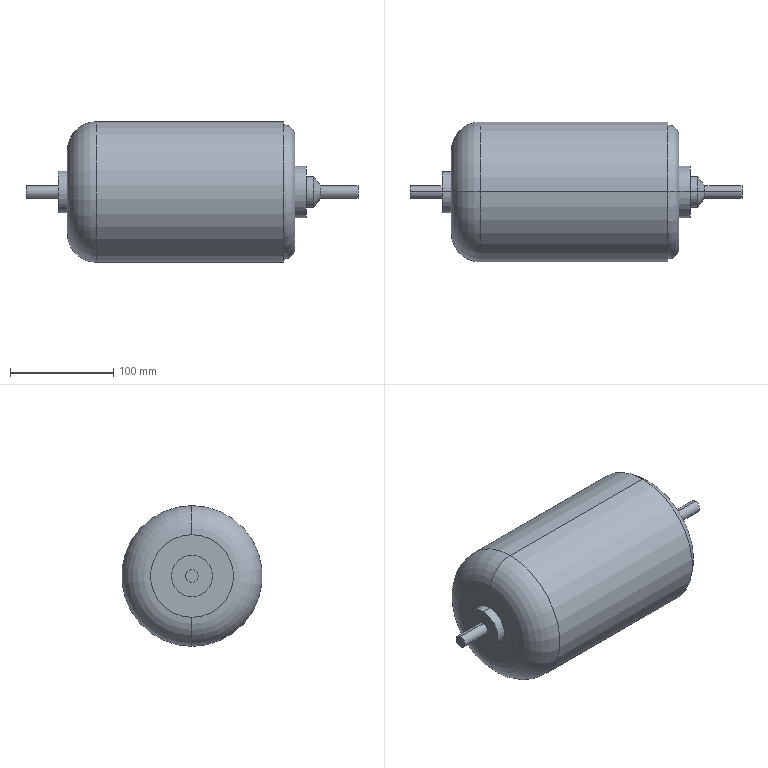Part | NX | features BREP 1 | 1 solid | 35 faces | box 321 x 136 x 136 mm | volume 3154531 mm3 | cylinder 16 | plane 13 | torus 4 | cone 2 | commonest cylinder face diameters 3 x4 12 x4 30 x2 40 x2 50 x2 136 x2
STEP:
#1=CARTESIAN_POINT('',(184.,0.,20.));
#2=VERTEX_POINT('',#1);
#3=CARTESIAN_POINT('',(184.,0.,-20.));
#4=VERTEX_POINT('',#3);
#5=CARTESIAN_POINT('',(184.,0.,0.));
#6=DIRECTION('',(-1.,0.,0.));
#7=DIRECTION('',(0.,0.,1.));
#8=AXIS2_PLACEMENT_3D('',#5,#6,#7);
#9=CIRCLE('',#8,20.);
#10=EDGE_CURVE('',#2,#4,#9,.T.);
#11=ORIENTED_EDGE('',*,*,#10,.T.);
#12=CARTESIAN_POINT('',(175.,0.,-20.));
#13=VERTEX_POINT('',#12);
#14=CARTESIAN_POINT('',(144.,0.,-20.));
#15=DIRECTION('',(-1.,0.,0.));
#16=VECTOR('',#15,1000.);
#17=LINE('',#14,#16);
#18=EDGE_CURVE('',#4,#13,#17,.T.);
#19=ORIENTED_EDGE('',*,*,#18,.T.);
#20=CARTESIAN_POINT('',(175.,0.,20.));
#21=VERTEX_POINT('',#20);
#22=CARTESIAN_POINT('',(175.,0.,0.));
#23=DIRECTION('',(-1.,0.,0.));
#24=DIRECTION('',(0.,0.,1.));
#25=AXIS2_PLACEMENT_3D('',#22,#23,#24);
#26=CIRCLE('',#25,20.);
#27=EDGE_CURVE('',#21,#13,#26,.T.);
#28=ORIENTED_EDGE('',*,*,#27,.F.);
#29=CARTESIAN_POINT('',(144.,0.,20.));
#30=DIRECTION('',(-1.,0.,0.));
#31=VECTOR('',#30,1000.);
#32=LINE('',#29,#31);
#33=EDGE_CURVE('',#2,#21,#32,.T.);
#34=ORIENTED_EDGE('',*,*,#33,.F.);
#35=EDGE_LOOP('',(#11,#19,#28,#34));
#36=FACE_BOUND('',#35,.T.);
#37=CARTESIAN_POINT('',(144.,0.,0.));
#38=DIRECTION('',(-1.,0.,0.));
#39=DIRECTION('',(0.,0.,-1.));
#40=AXIS2_PLACEMENT_3D('',#37,#38,#39);
#41=CYLINDRICAL_SURFACE('',#40,20.);
#42=ADVANCED_FACE('',(#36),#41,.T.);
#43=CARTESIAN_POINT('',(175.,0.,6.));
#44=VERTEX_POINT('',#43);
#45=CARTESIAN_POINT('',(175.,0.,-6.));
#46=VERTEX_POINT('',#45);
#47=CARTESIAN_POINT('',(175.,0.,0.));
#48=DIRECTION('',(-1.,0.,0.));
#49=DIRECTION('',(0.,0.,1.));
#50=AXIS2_PLACEMENT_3D('',#47,#48,#49);
#51=CIRCLE('',#50,6.);
#52=EDGE_CURVE('',#44,#46,#51,.T.);
#53=ORIENTED_EDGE('',*,*,#52,.T.);
#54=CARTESIAN_POINT('',(144.,0.,-6.));
#55=VERTEX_POINT('',#54);
#56=CARTESIAN_POINT('',(144.,0.,-6.));
#57=DIRECTION('',(-1.,0.,0.));
#58=VECTOR('',#57,1000.);
#59=LINE('',#56,#58);
#60=EDGE_CURVE('',#46,#55,#59,.T.);
#61=ORIENTED_EDGE('',*,*,#60,.T.);
#62=CARTESIAN_POINT('',(144.,0.,6.));
#63=VERTEX_POINT('',#62);
#64=CARTESIAN_POINT('',(144.,0.,0.));
#65=DIRECTION('',(-1.,0.,0.));
#66=DIRECTION('',(0.,0.,1.));
#67=AXIS2_PLACEMENT_3D('',#64,#65,#66);
#68=CIRCLE('',#67,6.);
#69=EDGE_CURVE('',#63,#55,#68,.T.);
#70=ORIENTED_EDGE('',*,*,#69,.F.);
#71=CARTESIAN_POINT('',(144.,0.,6.));
#72=DIRECTION('',(-1.,0.,0.));
#73=VECTOR('',#72,1000.);
#74=LINE('',#71,#73);
#75=EDGE_CURVE('',#44,#63,#74,.T.);
#76=ORIENTED_EDGE('',*,*,#75,.F.);
#77=EDGE_LOOP('',(#53,#61,#70,#76));
#78=FACE_BOUND('',#77,.T.);
#79=CARTESIAN_POINT('',(156.,5.809,-1.5));
#80=VERTEX_POINT('',#79);
#81=CARTESIAN_POINT('',(164.,5.809,-1.5));
#82=VERTEX_POINT('',#81);
#83=CARTESIAN_POINT('',(144.,5.809,-1.5));
#84=DIRECTION('',(1.,0.,0.));
#85=VECTOR('',#84,1000.);
#86=LINE('',#83,#85);
#87=EDGE_CURVE('',#80,#82,#86,.T.);
#88=ORIENTED_EDGE('',*,*,#87,.T.);
#89=CARTESIAN_POINT('',(164.,5.809,1.5));
#90=VERTEX_POINT('',#89);
#91=CARTESIAN_POINT('',(164.,5.809,-1.5));
#92=CARTESIAN_POINT('',(164.398,5.809,-1.5));
#93=CARTESIAN_POINT('',(165.172,5.906,-1.175));
#94=CARTESIAN_POINT('',(165.664,6.047,-0.002103));
#95=CARTESIAN_POINT('',(165.173,5.906,1.175));
#96=CARTESIAN_POINT('',(164.398,5.809,1.5));
#97=CARTESIAN_POINT('',(164.,5.809,1.5));
#98=B_SPLINE_CURVE_WITH_KNOTS('',3,(#91,#92,#93,#94,#95,#96,#97),.UNSPECIFIED.,.F.,.F.,(4,1,1,1,4),(0.,0.001177,0.002353,0.00353,0.004707),.UNSPECIFIED.);
#99=EDGE_CURVE('',#82,#90,#98,.T.);
#100=ORIENTED_EDGE('',*,*,#99,.T.);
#101=CARTESIAN_POINT('',(156.,5.809,1.5));
#102=VERTEX_POINT('',#101);
#103=CARTESIAN_POINT('',(144.,5.809,1.5));
#104=DIRECTION('',(-1.,0.,0.));
#105=VECTOR('',#104,1000.);
#106=LINE('',#103,#105);
#107=EDGE_CURVE('',#90,#102,#106,.T.);
#108=ORIENTED_EDGE('',*,*,#107,.T.);
#109=CARTESIAN_POINT('',(156.,5.809,1.5));
#110=CARTESIAN_POINT('',(155.602,5.809,1.5));
#111=CARTESIAN_POINT('',(154.828,5.906,1.175));
#112=CARTESIAN_POINT('',(154.336,6.047,0.002103));
#113=CARTESIAN_POINT('',(154.827,5.906,-1.175));
#114=CARTESIAN_POINT('',(155.602,5.809,-1.5));
#115=CARTESIAN_POINT('',(156.,5.809,-1.5));
#116=B_SPLINE_CURVE_WITH_KNOTS('',3,(#109,#110,#111,#112,#113,#114,#115),.UNSPECIFIED.,.F.,.F.,(4,1,1,1,4),(0.,0.001177,0.002353,0.00353,0.004707),.UNSPECIFIED.);
#117=EDGE_CURVE('',#102,#80,#116,.T.);
#118=ORIENTED_EDGE('',*,*,#117,.T.);
#119=EDGE_LOOP('',(#88,#100,#108,#118));
#120=FACE_BOUND('',#119,.T.);
#121=CARTESIAN_POINT('',(144.,0.,0.));
#122=DIRECTION('',(-1.,0.,0.));
#123=DIRECTION('',(0.,0.,-1.));
#124=AXIS2_PLACEMENT_3D('',#121,#122,#123);
#125=CYLINDRICAL_SURFACE('',#124,6.);
#126=ADVANCED_FACE('',(#78,#120),#125,.T.);
#127=CARTESIAN_POINT('',(465.,0.,6.));
#128=VERTEX_POINT('',#127);
#129=CARTESIAN_POINT('',(465.,0.,-6.));
#130=VERTEX_POINT('',#129);
#131=CARTESIAN_POINT('',(465.,0.,0.));
#132=DIRECTION('',(-1.,0.,0.));
#133=DIRECTION('',(0.,0.,1.));
#134=AXIS2_PLACEMENT_3D('',#131,#132,#133);
#135=CIRCLE('',#134,6.);
#136=EDGE_CURVE('',#128,#130,#135,.T.);
#137=ORIENTED_EDGE('',*,*,#136,.T.);
#138=CARTESIAN_POINT('',(429.,0.,-6.));
#139=VERTEX_POINT('',#138);
#140=CARTESIAN_POINT('',(144.,0.,-6.));
#141=DIRECTION('',(-1.,0.,0.));
#142=VECTOR('',#141,1000.);
#143=LINE('',#140,#142);
#144=EDGE_CURVE('',#130,#139,#143,.T.);
#145=ORIENTED_EDGE('',*,*,#144,.T.);
#146=CARTESIAN_POINT('',(429.,0.,6.));
#147=VERTEX_POINT('',#146);
#148=CARTESIAN_POINT('',(429.,0.,0.));
#149=DIRECTION('',(-1.,0.,0.));
#150=DIRECTION('',(0.,0.,1.));
#151=AXIS2_PLACEMENT_3D('',#148,#149,#150);
#152=CIRCLE('',#151,6.);
#153=EDGE_CURVE('',#147,#139,#152,.T.);
#154=ORIENTED_EDGE('',*,*,#153,.F.);
#155=CARTESIAN_POINT('',(144.,0.,6.));
#156=DIRECTION('',(-1.,0.,0.));
#157=VECTOR('',#156,1000.);
#158=LINE('',#155,#157);
#159=EDGE_CURVE('',#128,#147,#158,.T.);
#160=ORIENTED_EDGE('',*,*,#159,.F.);
#161=EDGE_LOOP('',(#137,#145,#154,#160));
#162=FACE_BOUND('',#161,.T.);
#163=CARTESIAN_POINT('',(444.,5.809,-1.5));
#164=VERTEX_POINT('',#163);
#165=CARTESIAN_POINT('',(452.,5.809,-1.5));
#166=VERTEX_POINT('',#165);
#167=CARTESIAN_POINT('',(144.,5.809,-1.5));
#168=DIRECTION('',(1.,0.,0.));
#169=VECTOR('',#168,1000.);
#170=LINE('',#167,#169);
#171=EDGE_CURVE('',#164,#166,#170,.T.);
#172=ORIENTED_EDGE('',*,*,#171,.T.);
#173=CARTESIAN_POINT('',(452.,5.809,1.5));
#174=VERTEX_POINT('',#173);
#175=CARTESIAN_POINT('',(452.,5.809,-1.5));
#176=CARTESIAN_POINT('',(452.398,5.809,-1.5));
#177=CARTESIAN_POINT('',(453.172,5.906,-1.175));
#178=CARTESIAN_POINT('',(453.664,6.047,-0.002103));
#179=CARTESIAN_POINT('',(453.173,5.906,1.175));
#180=CARTESIAN_POINT('',(452.398,5.809,1.5));
#181=CARTESIAN_POINT('',(452.,5.809,1.5));
#182=B_SPLINE_CURVE_WITH_KNOTS('',3,(#175,#176,#177,#178,#179,#180,#181),.UNSPECIFIED.,.F.,.F.,(4,1,1,1,4),(0.,0.001177,0.002353,0.00353,0.004707),.UNSPECIFIED.);
#183=EDGE_CURVE('',#166,#174,#182,.T.);
#184=ORIENTED_EDGE('',*,*,#183,.T.);
#185=CARTESIAN_POINT('',(444.,5.809,1.5));
#186=VERTEX_POINT('',#185);
#187=CARTESIAN_POINT('',(144.,5.809,1.5));
#188=DIRECTION('',(-1.,0.,0.));
#189=VECTOR('',#188,1000.);
#190=LINE('',#187,#189);
#191=EDGE_CURVE('',#174,#186,#190,.T.);
#192=ORIENTED_EDGE('',*,*,#191,.T.);
#193=CARTESIAN_POINT('',(444.,5.809,1.5));
#194=CARTESIAN_POINT('',(443.602,5.809,1.5));
#195=CARTESIAN_POINT('',(442.828,5.906,1.175));
#196=CARTESIAN_POINT('',(442.336,6.047,0.002103));
#197=CARTESIAN_POINT('',(442.827,5.906,-1.175));
#198=CARTESIAN_POINT('',(443.602,5.809,-1.5));
#199=CARTESIAN_POINT('',(444.,5.809,-1.5));
#200=B_SPLINE_CURVE_WITH_KNOTS('',3,(#193,#194,#195,#196,#197,#198,#199),.UNSPECIFIED.,.F.,.F.,(4,1,1,1,4),(0.,0.001177,0.002353,0.00353,0.004707),.UNSPECIFIED.);
#201=EDGE_CURVE('',#186,#164,#200,.T.);
#202=ORIENTED_EDGE('',*,*,#201,.T.);
#203=EDGE_LOOP('',(#172,#184,#192,#202));
#204=FACE_BOUND('',#203,.T.);
#205=CARTESIAN_POINT('',(144.,0.,0.));
#206=DIRECTION('',(-1.,0.,0.));
#207=DIRECTION('',(0.,0.,-1.));
#208=AXIS2_PLACEMENT_3D('',#205,#206,#207);
#209=CYLINDRICAL_SURFACE('',#208,6.);
#210=ADVANCED_FACE('',(#162,#204),#209,.T.);
#211=ORIENTED_EDGE('',*,*,#153,.T.);
#212=CARTESIAN_POINT('',(422.,0.,-15.));
#213=VERTEX_POINT('',#212);
#214=CARTESIAN_POINT('',(429.,0.,-6.));
#215=DIRECTION('',(-0.6139,0.,-0.7894));
#216=VECTOR('',#215,1000.);
#217=LINE('',#214,#216);
#218=EDGE_CURVE('',#139,#213,#217,.T.);
#219=ORIENTED_EDGE('',*,*,#218,.T.);
#220=CARTESIAN_POINT('',(422.,0.,15.));
#221=VERTEX_POINT('',#220);
#222=CARTESIAN_POINT('',(422.,0.,0.));
#223=DIRECTION('',(-1.,0.,0.));
#224=DIRECTION('',(0.,0.,1.));
#225=AXIS2_PLACEMENT_3D('',#222,#223,#224);
#226=CIRCLE('',#225,15.);
#227=EDGE_CURVE('',#221,#213,#226,.T.);
#228=ORIENTED_EDGE('',*,*,#227,.F.);
#229=CARTESIAN_POINT('',(429.,0.,6.));
#230=DIRECTION('',(-0.6139,0.,0.7894));
#231=VECTOR('',#230,1000.);
#232=LINE('',#229,#231);
#233=EDGE_CURVE('',#147,#221,#232,.T.);
#234=ORIENTED_EDGE('',*,*,#233,.F.);
#235=EDGE_LOOP('',(#211,#219,#228,#234));
#236=FACE_BOUND('',#235,.T.);
#237=CARTESIAN_POINT('',(429.,0.,0.));
#238=DIRECTION('',(-1.,0.,0.));
#239=DIRECTION('',(0.,0.,-1.));
#240=AXIS2_PLACEMENT_3D('',#237,#238,#239);
#241=CONICAL_SURFACE('',#240,6.,0.9098);
#242=ADVANCED_FACE('',(#236),#241,.T.);
#243=ORIENTED_EDGE('',*,*,#227,.T.);
#244=CARTESIAN_POINT('',(415.,0.,-15.));
#245=VERTEX_POINT('',#244);
#246=CARTESIAN_POINT('',(144.,0.,-15.));
#247=DIRECTION('',(-1.,0.,0.));
#248=VECTOR('',#247,1000.);
#249=LINE('',#246,#248);
#250=EDGE_CURVE('',#213,#245,#249,.T.);
#251=ORIENTED_EDGE('',*,*,#250,.T.);
#252=CARTESIAN_POINT('',(415.,0.,15.));
#253=VERTEX_POINT('',#252);
#254=CARTESIAN_POINT('',(415.,0.,0.));
#255=DIRECTION('',(-1.,0.,0.));
#256=DIRECTION('',(0.,0.,1.));
#257=AXIS2_PLACEMENT_3D('',#254,#255,#256);
#258=CIRCLE('',#257,15.);
#259=EDGE_CURVE('',#253,#245,#258,.T.);
#260=ORIENTED_EDGE('',*,*,#259,.F.);
#261=CARTESIAN_POINT('',(144.,0.,15.));
#262=DIRECTION('',(-1.,0.,0.));
#263=VECTOR('',#262,1000.);
#264=LINE('',#261,#263);
#265=EDGE_CURVE('',#221,#253,#264,.T.);
#266=ORIENTED_EDGE('',*,*,#265,.F.);
#267=EDGE_LOOP('',(#243,#251,#260,#266));
#268=FACE_BOUND('',#267,.T.);
#269=CARTESIAN_POINT('',(144.,0.,0.));
#270=DIRECTION('',(-1.,0.,0.));
#271=DIRECTION('',(0.,0.,-1.));
#272=AXIS2_PLACEMENT_3D('',#269,#270,#271);
#273=CYLINDRICAL_SURFACE('',#272,15.);
#274=ADVANCED_FACE('',(#268),#273,.T.);
#275=CARTESIAN_POINT('',(415.,0.,25.));
#276=VERTEX_POINT('',#275);
#277=CARTESIAN_POINT('',(415.,0.,-25.));
#278=VERTEX_POINT('',#277);
#279=CARTESIAN_POINT('',(415.,0.,0.));
#280=DIRECTION('',(-1.,0.,0.));
#281=DIRECTION('',(0.,0.,1.));
#282=AXIS2_PLACEMENT_3D('',#279,#280,#281);
#283=CIRCLE('',#282,25.);
#284=EDGE_CURVE('',#276,#278,#283,.T.);
#285=ORIENTED_EDGE('',*,*,#284,.T.);
#286=CARTESIAN_POINT('',(404.,0.,-25.));
#287=VERTEX_POINT('',#286);
#288=CARTESIAN_POINT('',(144.,0.,-25.));
#289=DIRECTION('',(-1.,0.,0.));
#290=VECTOR('',#289,1000.);
#291=LINE('',#288,#290);
#292=EDGE_CURVE('',#278,#287,#291,.T.);
#293=ORIENTED_EDGE('',*,*,#292,.T.);
#294=CARTESIAN_POINT('',(404.,0.,25.));
#295=VERTEX_POINT('',#294);
#296=CARTESIAN_POINT('',(404.,0.,0.));
#297=DIRECTION('',(-1.,0.,0.));
#298=DIRECTION('',(0.,0.,1.));
#299=AXIS2_PLACEMENT_3D('',#296,#297,#298);
#300=CIRCLE('',#299,25.);
#301=EDGE_CURVE('',#295,#287,#300,.T.);
#302=ORIENTED_EDGE('',*,*,#301,.F.);
#303=CARTESIAN_POINT('',(144.,0.,25.));
#304=DIRECTION('',(-1.,0.,0.));
#305=VECTOR('',#304,1000.);
#306=LINE('',#303,#305);
#307=EDGE_CURVE('',#276,#295,#306,.T.);
#308=ORIENTED_EDGE('',*,*,#307,.F.);
#309=EDGE_LOOP('',(#285,#293,#302,#308));
#310=FACE_BOUND('',#309,.T.);
#311=CARTESIAN_POINT('',(144.,0.,0.));
#312=DIRECTION('',(-1.,0.,0.));
#313=DIRECTION('',(0.,0.,-1.));
#314=AXIS2_PLACEMENT_3D('',#311,#312,#313);
#315=CYLINDRICAL_SURFACE('',#314,25.);
#316=ADVANCED_FACE('',(#310),#315,.T.);
#317=CARTESIAN_POINT('',(404.,0.,54.));
#318=VERTEX_POINT('',#317);
#319=CARTESIAN_POINT('',(404.,0.,-54.));
#320=VERTEX_POINT('',#319);
#321=CARTESIAN_POINT('',(404.,0.,0.));
#322=DIRECTION('',(-1.,0.,0.));
#323=DIRECTION('',(0.,0.,1.));
#324=AXIS2_PLACEMENT_3D('',#321,#322,#323);
#325=CIRCLE('',#324,54.);
#326=EDGE_CURVE('',#318,#320,#325,.T.);
#327=ORIENTED_EDGE('',*,*,#326,.T.);
#328=CARTESIAN_POINT('',(393.,0.,-65.));
#329=VERTEX_POINT('',#328);
#330=CARTESIAN_POINT('',(393.,0.,-54.));
#331=DIRECTION('',(0.,1.,0.));
#332=DIRECTION('',(0.,0.,1.));
#333=AXIS2_PLACEMENT_3D('',#330,#331,#332);
#334=CIRCLE('',#333,11.);
#335=EDGE_CURVE('',#320,#329,#334,.T.);
#336=ORIENTED_EDGE('',*,*,#335,.T.);
#337=CARTESIAN_POINT('',(393.,0.,65.));
#338=VERTEX_POINT('',#337);
#339=CARTESIAN_POINT('',(393.,0.,0.));
#340=DIRECTION('',(-1.,0.,0.));
#341=DIRECTION('',(0.,0.,1.));
#342=AXIS2_PLACEMENT_3D('',#339,#340,#341);
#343=CIRCLE('',#342,65.);
#344=EDGE_CURVE('',#338,#329,#343,.T.);
#345=ORIENTED_EDGE('',*,*,#344,.F.);
#346=CARTESIAN_POINT('',(393.,0.,54.));
#347=DIRECTION('',(0.,-1.,0.));
#348=DIRECTION('',(0.,0.,-1.));
#349=AXIS2_PLACEMENT_3D('',#346,#347,#348);
#350=CIRCLE('',#349,11.);
#351=EDGE_CURVE('',#318,#338,#350,.T.);
#352=ORIENTED_EDGE('',*,*,#351,.F.);
#353=EDGE_LOOP('',(#327,#336,#345,#352));
#354=FACE_BOUND('',#353,.T.);
#355=CARTESIAN_POINT('',(393.,0.,0.));
#356=DIRECTION('',(-1.,0.,0.));
#357=DIRECTION('',(0.,0.,-1.));
#358=AXIS2_PLACEMENT_3D('',#355,#356,#357);
#359=TOROIDAL_SURFACE('',#358,54.,11.);
#360=ADVANCED_FACE('',(#354),#359,.T.);
#361=CARTESIAN_POINT('',(393.,0.,68.));
#362=VERTEX_POINT('',#361);
#363=CARTESIAN_POINT('',(393.,0.,-68.));
#364=VERTEX_POINT('',#363);
#365=CARTESIAN_POINT('',(393.,0.,0.));
#366=DIRECTION('',(-1.,0.,0.));
#367=DIRECTION('',(0.,0.,1.));
#368=AXIS2_PLACEMENT_3D('',#365,#366,#367);
#369=CIRCLE('',#368,68.);
#370=EDGE_CURVE('',#362,#364,#369,.T.);
#371=ORIENTED_EDGE('',*,*,#370,.T.);
#372=CARTESIAN_POINT('',(212.,0.,-68.));
#373=VERTEX_POINT('',#372);
#374=CARTESIAN_POINT('',(144.,0.,-68.));
#375=DIRECTION('',(-1.,0.,0.));
#376=VECTOR('',#375,1000.);
#377=LINE('',#374,#376);
#378=EDGE_CURVE('',#364,#373,#377,.T.);
#379=ORIENTED_EDGE('',*,*,#378,.T.);
#380=CARTESIAN_POINT('',(212.,0.,68.));
#381=VERTEX_POINT('',#380);
#382=CARTESIAN_POINT('',(212.,0.,0.));
#383=DIRECTION('',(-1.,0.,0.));
#384=DIRECTION('',(0.,0.,1.));
#385=AXIS2_PLACEMENT_3D('',#382,#383,#384);
#386=CIRCLE('',#385,68.);
#387=EDGE_CURVE('',#381,#373,#386,.T.);
#388=ORIENTED_EDGE('',*,*,#387,.F.);
#389=CARTESIAN_POINT('',(144.,0.,68.));
#390=DIRECTION('',(-1.,0.,0.));
#391=VECTOR('',#390,1000.);
#392=LINE('',#389,#391);
#393=EDGE_CURVE('',#362,#381,#392,.T.);
#394=ORIENTED_EDGE('',*,*,#393,.F.);
#395=EDGE_LOOP('',(#371,#379,#388,#394));
#396=FACE_BOUND('',#395,.T.);
#397=CARTESIAN_POINT('',(144.,0.,0.));
#398=DIRECTION('',(-1.,0.,0.));
#399=DIRECTION('',(0.,0.,-1.));
#400=AXIS2_PLACEMENT_3D('',#397,#398,#399);
#401=CYLINDRICAL_SURFACE('',#400,68.);
#402=ADVANCED_FACE('',(#396),#401,.T.);
#403=ORIENTED_EDGE('',*,*,#387,.T.);
#404=CARTESIAN_POINT('',(184.,0.,-40.));
#405=VERTEX_POINT('',#404);
#406=CARTESIAN_POINT('',(212.,0.,-40.));
#407=DIRECTION('',(0.,1.,0.));
#408=DIRECTION('',(0.,0.,1.));
#409=AXIS2_PLACEMENT_3D('',#406,#407,#408);
#410=CIRCLE('',#409,28.);
#411=EDGE_CURVE('',#373,#405,#410,.T.);
#412=ORIENTED_EDGE('',*,*,#411,.T.);
#413=CARTESIAN_POINT('',(184.,0.,40.));
#414=VERTEX_POINT('',#413);
#415=CARTESIAN_POINT('',(184.,0.,0.));
#416=DIRECTION('',(-1.,0.,0.));
#417=DIRECTION('',(0.,0.,1.));
#418=AXIS2_PLACEMENT_3D('',#415,#416,#417);
#419=CIRCLE('',#418,40.);
#420=EDGE_CURVE('',#414,#405,#419,.T.);
#421=ORIENTED_EDGE('',*,*,#420,.F.);
#422=CARTESIAN_POINT('',(212.,0.,40.));
#423=DIRECTION('',(0.,-1.,0.));
#424=DIRECTION('',(0.,0.,-1.));
#425=AXIS2_PLACEMENT_3D('',#422,#423,#424);
#426=CIRCLE('',#425,28.);
#427=EDGE_CURVE('',#381,#414,#426,.T.);
#428=ORIENTED_EDGE('',*,*,#427,.F.);
#429=EDGE_LOOP('',(#403,#412,#421,#428));
#430=FACE_BOUND('',#429,.T.);
#431=CARTESIAN_POINT('',(212.,0.,0.));
#432=DIRECTION('',(-1.,0.,0.));
#433=DIRECTION('',(0.,0.,-1.));
#434=AXIS2_PLACEMENT_3D('',#431,#432,#433);
#435=TOROIDAL_SURFACE('',#434,40.,28.);
#436=ADVANCED_FACE('',(#430),#435,.T.);
#437=ORIENTED_EDGE('',*,*,#411,.F.);
#438=CARTESIAN_POINT('',(212.,0.,0.));
#439=DIRECTION('',(-1.,0.,0.));
#440=DIRECTION('',(0.,0.,1.));
#441=AXIS2_PLACEMENT_3D('',#438,#439,#440);
#442=CIRCLE('',#441,68.);
#443=EDGE_CURVE('',#373,#381,#442,.T.);
#444=ORIENTED_EDGE('',*,*,#443,.T.);
#445=ORIENTED_EDGE('',*,*,#427,.T.);
#446=CARTESIAN_POINT('',(184.,0.,0.));
#447=DIRECTION('',(-1.,0.,0.));
#448=DIRECTION('',(0.,0.,1.));
#449=AXIS2_PLACEMENT_3D('',#446,#447,#448);
#450=CIRCLE('',#449,40.);
#451=EDGE_CURVE('',#405,#414,#450,.T.);
#452=ORIENTED_EDGE('',*,*,#451,.F.);
#453=EDGE_LOOP('',(#437,#444,#445,#452));
#454=FACE_BOUND('',#453,.T.);
#455=CARTESIAN_POINT('',(212.,0.,0.));
#456=DIRECTION('',(-1.,0.,0.));
#457=DIRECTION('',(0.,0.,-1.));
#458=AXIS2_PLACEMENT_3D('',#455,#456,#457);
#459=TOROIDAL_SURFACE('',#458,40.,28.);
#460=ADVANCED_FACE('',(#454),#459,.T.);
#461=ORIENTED_EDGE('',*,*,#378,.F.);
#462=CARTESIAN_POINT('',(393.,0.,0.));
#463=DIRECTION('',(-1.,0.,0.));
#464=DIRECTION('',(0.,0.,1.));
#465=AXIS2_PLACEMENT_3D('',#462,#463,#464);
#466=CIRCLE('',#465,68.);
#467=EDGE_CURVE('',#364,#362,#466,.T.);
#468=ORIENTED_EDGE('',*,*,#467,.T.);
#469=ORIENTED_EDGE('',*,*,#393,.T.);
#470=ORIENTED_EDGE('',*,*,#443,.F.);
#471=EDGE_LOOP('',(#461,#468,#469,#470));
#472=FACE_BOUND('',#471,.T.);
#473=CARTESIAN_POINT('',(144.,0.,0.));
#474=DIRECTION('',(-1.,0.,0.));
#475=DIRECTION('',(0.,0.,-1.));
#476=AXIS2_PLACEMENT_3D('',#473,#474,#475);
#477=CYLINDRICAL_SURFACE('',#476,68.);
#478=ADVANCED_FACE('',(#472),#477,.T.);
#479=ORIENTED_EDGE('',*,*,#370,.F.);
#480=ORIENTED_EDGE('',*,*,#467,.F.);
#481=EDGE_LOOP('',(#479,#480));
#482=FACE_BOUND('',#481,.T.);
#483=ORIENTED_EDGE('',*,*,#344,.T.);
#484=CARTESIAN_POINT('',(393.,0.,0.));
#485=DIRECTION('',(-1.,0.,0.));
#486=DIRECTION('',(0.,0.,1.));
#487=AXIS2_PLACEMENT_3D('',#484,#485,#486);
#488=CIRCLE('',#487,65.);
#489=EDGE_CURVE('',#329,#338,#488,.T.);
#490=ORIENTED_EDGE('',*,*,#489,.T.);
#491=EDGE_LOOP('',(#483,#490));
#492=FACE_BOUND('',#491,.T.);
#493=CARTESIAN_POINT('',(393.,68.,0.));
#494=DIRECTION('',(-1.,0.,0.));
#495=DIRECTION('',(0.,0.,-1.));
#496=AXIS2_PLACEMENT_3D('',#493,#494,#495);
#497=PLANE('',#496);
#498=ADVANCED_FACE('',(#482,#492),#497,.F.);
#499=ORIENTED_EDGE('',*,*,#335,.F.);
#500=CARTESIAN_POINT('',(404.,0.,0.));
#501=DIRECTION('',(-1.,0.,0.));
#502=DIRECTION('',(0.,0.,1.));
#503=AXIS2_PLACEMENT_3D('',#500,#501,#502);
#504=CIRCLE('',#503,54.);
#505=EDGE_CURVE('',#320,#318,#504,.T.);
#506=ORIENTED_EDGE('',*,*,#505,.T.);
#507=ORIENTED_EDGE('',*,*,#351,.T.);
#508=ORIENTED_EDGE('',*,*,#489,.F.);
#509=EDGE_LOOP('',(#499,#506,#507,#508));
#510=FACE_BOUND('',#509,.T.);
#511=CARTESIAN_POINT('',(393.,0.,0.));
#512=DIRECTION('',(-1.,0.,0.));
#513=DIRECTION('',(0.,0.,-1.));
#514=AXIS2_PLACEMENT_3D('',#511,#512,#513);
#515=TOROIDAL_SURFACE('',#514,54.,11.);
#516=ADVANCED_FACE('',(#510),#515,.T.);
#517=ORIENTED_EDGE('',*,*,#326,.F.);
#518=ORIENTED_EDGE('',*,*,#505,.F.);
#519=EDGE_LOOP('',(#517,#518));
#520=FACE_BOUND('',#519,.T.);
#521=ORIENTED_EDGE('',*,*,#301,.T.);
#522=CARTESIAN_POINT('',(404.,0.,0.));
#523=DIRECTION('',(-1.,0.,0.));
#524=DIRECTION('',(0.,0.,1.));
#525=AXIS2_PLACEMENT_3D('',#522,#523,#524);
#526=CIRCLE('',#525,25.);
#527=EDGE_CURVE('',#287,#295,#526,.T.);
#528=ORIENTED_EDGE('',*,*,#527,.T.);
#529=EDGE_LOOP('',(#521,#528));
#530=FACE_BOUND('',#529,.T.);
#531=CARTESIAN_POINT('',(404.,54.,0.));
#532=DIRECTION('',(-1.,0.,0.));
#533=DIRECTION('',(0.,0.,-1.));
#534=AXIS2_PLACEMENT_3D('',#531,#532,#533);
#535=PLANE('',#534);
#536=ADVANCED_FACE('',(#520,#530),#535,.F.);
#537=ORIENTED_EDGE('',*,*,#292,.F.);
#538=CARTESIAN_POINT('',(415.,0.,0.));
#539=DIRECTION('',(-1.,0.,0.));
#540=DIRECTION('',(0.,0.,1.));
#541=AXIS2_PLACEMENT_3D('',#538,#539,#540);
#542=CIRCLE('',#541,25.);
#543=EDGE_CURVE('',#278,#276,#542,.T.);
#544=ORIENTED_EDGE('',*,*,#543,.T.);
#545=ORIENTED_EDGE('',*,*,#307,.T.);
#546=ORIENTED_EDGE('',*,*,#527,.F.);
#547=EDGE_LOOP('',(#537,#544,#545,#546));
#548=FACE_BOUND('',#547,.T.);
#549=CARTESIAN_POINT('',(144.,0.,0.));
#550=DIRECTION('',(-1.,0.,0.));
#551=DIRECTION('',(0.,0.,-1.));
#552=AXIS2_PLACEMENT_3D('',#549,#550,#551);
#553=CYLINDRICAL_SURFACE('',#552,25.);
#554=ADVANCED_FACE('',(#548),#553,.T.);
#555=ORIENTED_EDGE('',*,*,#284,.F.);
#556=ORIENTED_EDGE('',*,*,#543,.F.);
#557=EDGE_LOOP('',(#555,#556));
#558=FACE_BOUND('',#557,.T.);
#559=ORIENTED_EDGE('',*,*,#259,.T.);
#560=CARTESIAN_POINT('',(415.,0.,0.));
#561=DIRECTION('',(-1.,0.,0.));
#562=DIRECTION('',(0.,0.,1.));
#563=AXIS2_PLACEMENT_3D('',#560,#561,#562);
#564=CIRCLE('',#563,15.);
#565=EDGE_CURVE('',#245,#253,#564,.T.);
#566=ORIENTED_EDGE('',*,*,#565,.T.);
#567=EDGE_LOOP('',(#559,#566));
#568=FACE_BOUND('',#567,.T.);
#569=CARTESIAN_POINT('',(415.,25.,0.));
#570=DIRECTION('',(-1.,0.,0.));
#571=DIRECTION('',(0.,0.,-1.));
#572=AXIS2_PLACEMENT_3D('',#569,#570,#571);
#573=PLANE('',#572);
#574=ADVANCED_FACE('',(#558,#568),#573,.F.);
#575=ORIENTED_EDGE('',*,*,#250,.F.);
#576=CARTESIAN_POINT('',(422.,0.,0.));
#577=DIRECTION('',(-1.,0.,0.));
#578=DIRECTION('',(0.,0.,1.));
#579=AXIS2_PLACEMENT_3D('',#576,#577,#578);
#580=CIRCLE('',#579,15.);
#581=EDGE_CURVE('',#213,#221,#580,.T.);
#582=ORIENTED_EDGE('',*,*,#581,.T.);
#583=ORIENTED_EDGE('',*,*,#265,.T.);
#584=ORIENTED_EDGE('',*,*,#565,.F.);
#585=EDGE_LOOP('',(#575,#582,#583,#584));
#586=FACE_BOUND('',#585,.T.);
#587=CARTESIAN_POINT('',(144.,0.,0.));
#588=DIRECTION('',(-1.,0.,0.));
#589=DIRECTION('',(0.,0.,-1.));
#590=AXIS2_PLACEMENT_3D('',#587,#588,#589);
#591=CYLINDRICAL_SURFACE('',#590,15.);
#592=ADVANCED_FACE('',(#586),#591,.T.);
#593=ORIENTED_EDGE('',*,*,#218,.F.);
#594=CARTESIAN_POINT('',(429.,0.,0.));
#595=DIRECTION('',(-1.,0.,0.));
#596=DIRECTION('',(0.,0.,1.));
#597=AXIS2_PLACEMENT_3D('',#594,#595,#596);
#598=CIRCLE('',#597,6.);
#599=EDGE_CURVE('',#139,#147,#598,.T.);
#600=ORIENTED_EDGE('',*,*,#599,.T.);
#601=ORIENTED_EDGE('',*,*,#233,.T.);
#602=ORIENTED_EDGE('',*,*,#581,.F.);
#603=EDGE_LOOP('',(#593,#600,#601,#602));
#604=FACE_BOUND('',#603,.T.);
#605=CARTESIAN_POINT('',(429.,0.,0.));
#606=DIRECTION('',(-1.,0.,0.));
#607=DIRECTION('',(0.,0.,-1.));
#608=AXIS2_PLACEMENT_3D('',#605,#606,#607);
#609=CONICAL_SURFACE('',#608,6.,0.9098);
#610=ADVANCED_FACE('',(#604),#609,.T.);
#611=ORIENTED_EDGE('',*,*,#144,.F.);
#612=CARTESIAN_POINT('',(465.,0.,0.));
#613=DIRECTION('',(-1.,0.,0.));
#614=DIRECTION('',(0.,0.,1.));
#615=AXIS2_PLACEMENT_3D('',#612,#613,#614);
#616=CIRCLE('',#615,6.);
#617=EDGE_CURVE('',#130,#128,#616,.T.);
#618=ORIENTED_EDGE('',*,*,#617,.T.);
#619=ORIENTED_EDGE('',*,*,#159,.T.);
#620=ORIENTED_EDGE('',*,*,#599,.F.);
#621=EDGE_LOOP('',(#611,#618,#619,#620));
#622=FACE_BOUND('',#621,.T.);
#623=CARTESIAN_POINT('',(144.,0.,0.));
#624=DIRECTION('',(-1.,0.,0.));
#625=DIRECTION('',(0.,0.,-1.));
#626=AXIS2_PLACEMENT_3D('',#623,#624,#625);
#627=CYLINDRICAL_SURFACE('',#626,6.);
#628=ADVANCED_FACE('',(#622),#627,.T.);
#629=ORIENTED_EDGE('',*,*,#136,.F.);
#630=ORIENTED_EDGE('',*,*,#617,.F.);
#631=EDGE_LOOP('',(#629,#630));
#632=FACE_BOUND('',#631,.T.);
#633=CARTESIAN_POINT('',(465.,6.,0.));
#634=DIRECTION('',(-1.,0.,0.));
#635=DIRECTION('',(0.,0.,-1.));
#636=AXIS2_PLACEMENT_3D('',#633,#634,#635);
#637=PLANE('',#636);
#638=ADVANCED_FACE('',(#632),#637,.F.);
#639=ORIENTED_EDGE('',*,*,#69,.T.);
#640=CARTESIAN_POINT('',(144.,0.,0.));
#641=DIRECTION('',(-1.,0.,0.));
#642=DIRECTION('',(0.,0.,1.));
#643=AXIS2_PLACEMENT_3D('',#640,#641,#642);
#644=CIRCLE('',#643,6.);
#645=EDGE_CURVE('',#55,#63,#644,.T.);
#646=ORIENTED_EDGE('',*,*,#645,.T.);
#647=EDGE_LOOP('',(#639,#646));
#648=FACE_BOUND('',#647,.T.);
#649=CARTESIAN_POINT('',(144.,6.,0.));
#650=DIRECTION('',(1.,0.,0.));
#651=DIRECTION('',(0.,0.,-1.));
#652=AXIS2_PLACEMENT_3D('',#649,#650,#651);
#653=PLANE('',#652);
#654=ADVANCED_FACE('',(#648),#653,.F.);
#655=ORIENTED_EDGE('',*,*,#60,.F.);
#656=CARTESIAN_POINT('',(175.,0.,0.));
#657=DIRECTION('',(-1.,0.,0.));
#658=DIRECTION('',(0.,0.,1.));
#659=AXIS2_PLACEMENT_3D('',#656,#657,#658);
#660=CIRCLE('',#659,6.);
#661=EDGE_CURVE('',#46,#44,#660,.T.);
#662=ORIENTED_EDGE('',*,*,#661,.T.);
#663=ORIENTED_EDGE('',*,*,#75,.T.);
#664=ORIENTED_EDGE('',*,*,#645,.F.);
#665=EDGE_LOOP('',(#655,#662,#663,#664));
#666=FACE_BOUND('',#665,.T.);
#667=CARTESIAN_POINT('',(144.,0.,0.));
#668=DIRECTION('',(-1.,0.,0.));
#669=DIRECTION('',(0.,0.,-1.));
#670=AXIS2_PLACEMENT_3D('',#667,#668,#669);
#671=CYLINDRICAL_SURFACE('',#670,6.);
#672=ADVANCED_FACE('',(#666),#671,.T.);
#673=ORIENTED_EDGE('',*,*,#27,.T.);
#674=CARTESIAN_POINT('',(175.,0.,0.));
#675=DIRECTION('',(-1.,0.,0.));
#676=DIRECTION('',(0.,0.,1.));
#677=AXIS2_PLACEMENT_3D('',#674,#675,#676);
#678=CIRCLE('',#677,20.);
#679=EDGE_CURVE('',#13,#21,#678,.T.);
#680=ORIENTED_EDGE('',*,*,#679,.T.);
#681=EDGE_LOOP('',(#673,#680));
#682=FACE_BOUND('',#681,.T.);
#683=ORIENTED_EDGE('',*,*,#52,.F.);
#684=ORIENTED_EDGE('',*,*,#661,.F.);
#685=EDGE_LOOP('',(#683,#684));
#686=FACE_BOUND('',#685,.T.);
#687=CARTESIAN_POINT('',(175.,6.,0.));
#688=DIRECTION('',(1.,0.,0.));
#689=DIRECTION('',(0.,0.,-1.));
#690=AXIS2_PLACEMENT_3D('',#687,#688,#689);
#691=PLANE('',#690);
#692=ADVANCED_FACE('',(#682,#686),#691,.F.);
#693=ORIENTED_EDGE('',*,*,#18,.F.);
#694=CARTESIAN_POINT('',(184.,0.,0.));
#695=DIRECTION('',(-1.,0.,0.));
#696=DIRECTION('',(0.,0.,1.));
#697=AXIS2_PLACEMENT_3D('',#694,#695,#696);
#698=CIRCLE('',#697,20.);
#699=EDGE_CURVE('',#4,#2,#698,.T.);
#700=ORIENTED_EDGE('',*,*,#699,.T.);
#701=ORIENTED_EDGE('',*,*,#33,.T.);
#702=ORIENTED_EDGE('',*,*,#679,.F.);
#703=EDGE_LOOP('',(#693,#700,#701,#702));
#704=FACE_BOUND('',#703,.T.);
#705=CARTESIAN_POINT('',(144.,0.,0.));
#706=DIRECTION('',(-1.,0.,0.));
#707=DIRECTION('',(0.,0.,-1.));
#708=AXIS2_PLACEMENT_3D('',#705,#706,#707);
#709=CYLINDRICAL_SURFACE('',#708,20.);
#710=ADVANCED_FACE('',(#704),#709,.T.);
#711=ORIENTED_EDGE('',*,*,#420,.T.);
#712=ORIENTED_EDGE('',*,*,#451,.T.);
#713=EDGE_LOOP('',(#711,#712));
#714=FACE_BOUND('',#713,.T.);
#715=ORIENTED_EDGE('',*,*,#10,.F.);
#716=ORIENTED_EDGE('',*,*,#699,.F.);
#717=EDGE_LOOP('',(#715,#716));
#718=FACE_BOUND('',#717,.T.);
#719=CARTESIAN_POINT('',(184.,40.,0.));
#720=DIRECTION('',(1.,0.,0.));
#721=DIRECTION('',(0.,0.,-1.));
#722=AXIS2_PLACEMENT_3D('',#719,#720,#721);
#723=PLANE('',#722);
#724=ADVANCED_FACE('',(#714,#718),#723,.F.);
#725=CARTESIAN_POINT('',(444.,4.5,1.5));
#726=VERTEX_POINT('',#725);
#727=CARTESIAN_POINT('',(444.,4.5,1.5));
#728=DIRECTION('',(0.,1.,0.));
#729=VECTOR('',#728,1000.);
#730=LINE('',#727,#729);
#731=EDGE_CURVE('',#726,#186,#730,.T.);
#732=ORIENTED_EDGE('',*,*,#731,.F.);
#733=CARTESIAN_POINT('',(444.,4.5,-1.5));
#734=VERTEX_POINT('',#733);
#735=CARTESIAN_POINT('',(444.,4.5,0.));
#736=DIRECTION('',(0.,1.,0.));
#737=DIRECTION('',(0.,0.,1.));
#738=AXIS2_PLACEMENT_3D('',#735,#736,#737);
#739=CIRCLE('',#738,1.5);
#740=EDGE_CURVE('',#734,#726,#739,.T.);
#741=ORIENTED_EDGE('',*,*,#740,.F.);
#742=CARTESIAN_POINT('',(444.,4.5,-1.5));
#743=DIRECTION('',(0.,1.,0.));
#744=VECTOR('',#743,1000.);
#745=LINE('',#742,#744);
#746=EDGE_CURVE('',#734,#164,#745,.T.);
#747=ORIENTED_EDGE('',*,*,#746,.T.);
#748=ORIENTED_EDGE('',*,*,#201,.F.);
#749=EDGE_LOOP('',(#732,#741,#747,#748));
#750=FACE_BOUND('',#749,.T.);
#751=CARTESIAN_POINT('',(444.,4.5,0.));
#752=DIRECTION('',(0.,1.,0.));
#753=DIRECTION('',(0.,0.,-1.));
#754=AXIS2_PLACEMENT_3D('',#751,#752,#753);
#755=CYLINDRICAL_SURFACE('',#754,1.5);
#756=ADVANCED_FACE('',(#750),#755,.F.);
#757=ORIENTED_EDGE('',*,*,#746,.F.);
#758=CARTESIAN_POINT('',(452.,4.5,-1.5));
#759=VERTEX_POINT('',#758);
#760=CARTESIAN_POINT('',(444.,4.5,-1.5));
#761=DIRECTION('',(-1.,0.,0.));
#762=VECTOR('',#761,1000.);
#763=LINE('',#760,#762);
#764=EDGE_CURVE('',#759,#734,#763,.T.);
#765=ORIENTED_EDGE('',*,*,#764,.F.);
#766=CARTESIAN_POINT('',(452.,4.5,-1.5));
#767=DIRECTION('',(0.,1.,0.));
#768=VECTOR('',#767,1000.);
#769=LINE('',#766,#768);
#770=EDGE_CURVE('',#759,#166,#769,.T.);
#771=ORIENTED_EDGE('',*,*,#770,.T.);
#772=ORIENTED_EDGE('',*,*,#171,.F.);
#773=EDGE_LOOP('',(#757,#765,#771,#772));
#774=FACE_BOUND('',#773,.T.);
#775=CARTESIAN_POINT('',(444.,4.5,-1.5));
#776=DIRECTION('',(0.,0.,-1.));
#777=DIRECTION('',(0.,1.,0.));
#778=AXIS2_PLACEMENT_3D('',#775,#776,#777);
#779=PLANE('',#778);
#780=ADVANCED_FACE('',(#774),#779,.F.);
#781=ORIENTED_EDGE('',*,*,#770,.F.);
#782=CARTESIAN_POINT('',(452.,4.5,1.5));
#783=VERTEX_POINT('',#782);
#784=CARTESIAN_POINT('',(452.,4.5,0.));
#785=DIRECTION('',(0.,1.,0.));
#786=DIRECTION('',(0.,0.,1.));
#787=AXIS2_PLACEMENT_3D('',#784,#785,#786);
#788=CIRCLE('',#787,1.5);
#789=EDGE_CURVE('',#783,#759,#788,.T.);
#790=ORIENTED_EDGE('',*,*,#789,.F.);
#791=CARTESIAN_POINT('',(452.,4.5,1.5));
#792=DIRECTION('',(0.,1.,0.));
#793=VECTOR('',#792,1000.);
#794=LINE('',#791,#793);
#795=EDGE_CURVE('',#783,#174,#794,.T.);
#796=ORIENTED_EDGE('',*,*,#795,.T.);
#797=ORIENTED_EDGE('',*,*,#183,.F.);
#798=EDGE_LOOP('',(#781,#790,#796,#797));
#799=FACE_BOUND('',#798,.T.);
#800=CARTESIAN_POINT('',(452.,4.5,0.));
#801=DIRECTION('',(0.,1.,0.));
#802=DIRECTION('',(0.,0.,-1.));
#803=AXIS2_PLACEMENT_3D('',#800,#801,#802);
#804=CYLINDRICAL_SURFACE('',#803,1.5);
#805=ADVANCED_FACE('',(#799),#804,.F.);
#806=ORIENTED_EDGE('',*,*,#795,.F.);
#807=CARTESIAN_POINT('',(444.,4.5,1.5));
#808=DIRECTION('',(1.,0.,0.));
#809=VECTOR('',#808,1000.);
#810=LINE('',#807,#809);
#811=EDGE_CURVE('',#726,#783,#810,.T.);
#812=ORIENTED_EDGE('',*,*,#811,.F.);
#813=ORIENTED_EDGE('',*,*,#731,.T.);
#814=ORIENTED_EDGE('',*,*,#191,.F.);
#815=EDGE_LOOP('',(#806,#812,#813,#814));
#816=FACE_BOUND('',#815,.T.);
#817=CARTESIAN_POINT('',(444.,4.5,1.5));
#818=DIRECTION('',(0.,0.,1.));
#819=DIRECTION('',(0.,1.,0.));
#820=AXIS2_PLACEMENT_3D('',#817,#818,#819);
#821=PLANE('',#820);
#822=ADVANCED_FACE('',(#816),#821,.F.);
#823=ORIENTED_EDGE('',*,*,#740,.T.);
#824=ORIENTED_EDGE('',*,*,#811,.T.);
#825=ORIENTED_EDGE('',*,*,#789,.T.);
#826=ORIENTED_EDGE('',*,*,#764,.T.);
#827=EDGE_LOOP('',(#823,#824,#825,#826));
#828=FACE_BOUND('',#827,.T.);
#829=CARTESIAN_POINT('',(444.,4.5,0.));
#830=DIRECTION('',(0.,1.,0.));
#831=DIRECTION('',(0.,0.,1.));
#832=AXIS2_PLACEMENT_3D('',#829,#830,#831);
#833=PLANE('',#832);
#834=ADVANCED_FACE('',(#828),#833,.T.);
#835=CARTESIAN_POINT('',(156.,4.5,1.5));
#836=VERTEX_POINT('',#835);
#837=CARTESIAN_POINT('',(156.,4.5,1.5));
#838=DIRECTION('',(0.,1.,0.));
#839=VECTOR('',#838,1000.);
#840=LINE('',#837,#839);
#841=EDGE_CURVE('',#836,#102,#840,.T.);
#842=ORIENTED_EDGE('',*,*,#841,.F.);
#843=CARTESIAN_POINT('',(156.,4.5,-1.5));
#844=VERTEX_POINT('',#843);
#845=CARTESIAN_POINT('',(156.,4.5,0.));
#846=DIRECTION('',(0.,1.,0.));
#847=DIRECTION('',(0.,0.,1.));
#848=AXIS2_PLACEMENT_3D('',#845,#846,#847);
#849=CIRCLE('',#848,1.5);
#850=EDGE_CURVE('',#844,#836,#849,.T.);
#851=ORIENTED_EDGE('',*,*,#850,.F.);
#852=CARTESIAN_POINT('',(156.,4.5,-1.5));
#853=DIRECTION('',(0.,1.,0.));
#854=VECTOR('',#853,1000.);
#855=LINE('',#852,#854);
#856=EDGE_CURVE('',#844,#80,#855,.T.);
#857=ORIENTED_EDGE('',*,*,#856,.T.);
#858=ORIENTED_EDGE('',*,*,#117,.F.);
#859=EDGE_LOOP('',(#842,#851,#857,#858));
#860=FACE_BOUND('',#859,.T.);
#861=CARTESIAN_POINT('',(156.,4.5,0.));
#862=DIRECTION('',(0.,1.,0.));
#863=DIRECTION('',(0.,0.,-1.));
#864=AXIS2_PLACEMENT_3D('',#861,#862,#863);
#865=CYLINDRICAL_SURFACE('',#864,1.5);
#866=ADVANCED_FACE('',(#860),#865,.F.);
#867=ORIENTED_EDGE('',*,*,#856,.F.);
#868=CARTESIAN_POINT('',(164.,4.5,-1.5));
#869=VERTEX_POINT('',#868);
#870=CARTESIAN_POINT('',(156.,4.5,-1.5));
#871=DIRECTION('',(-1.,0.,0.));
#872=VECTOR('',#871,1000.);
#873=LINE('',#870,#872);
#874=EDGE_CURVE('',#869,#844,#873,.T.);
#875=ORIENTED_EDGE('',*,*,#874,.F.);
#876=CARTESIAN_POINT('',(164.,4.5,-1.5));
#877=DIRECTION('',(0.,1.,0.));
#878=VECTOR('',#877,1000.);
#879=LINE('',#876,#878);
#880=EDGE_CURVE('',#869,#82,#879,.T.);
#881=ORIENTED_EDGE('',*,*,#880,.T.);
#882=ORIENTED_EDGE('',*,*,#87,.F.);
#883=EDGE_LOOP('',(#867,#875,#881,#882));
#884=FACE_BOUND('',#883,.T.);
#885=CARTESIAN_POINT('',(156.,4.5,-1.5));
#886=DIRECTION('',(0.,0.,-1.));
#887=DIRECTION('',(0.,1.,0.));
#888=AXIS2_PLACEMENT_3D('',#885,#886,#887);
#889=PLANE('',#888);
#890=ADVANCED_FACE('',(#884),#889,.F.);
#891=ORIENTED_EDGE('',*,*,#880,.F.);
#892=CARTESIAN_POINT('',(164.,4.5,1.5));
#893=VERTEX_POINT('',#892);
#894=CARTESIAN_POINT('',(164.,4.5,0.));
#895=DIRECTION('',(0.,1.,0.));
#896=DIRECTION('',(0.,0.,1.));
#897=AXIS2_PLACEMENT_3D('',#894,#895,#896);
#898=CIRCLE('',#897,1.5);
#899=EDGE_CURVE('',#893,#869,#898,.T.);
#900=ORIENTED_EDGE('',*,*,#899,.F.);
#901=CARTESIAN_POINT('',(164.,4.5,1.5));
#902=DIRECTION('',(0.,1.,0.));
#903=VECTOR('',#902,1000.);
#904=LINE('',#901,#903);
#905=EDGE_CURVE('',#893,#90,#904,.T.);
#906=ORIENTED_EDGE('',*,*,#905,.T.);
#907=ORIENTED_EDGE('',*,*,#99,.F.);
#908=EDGE_LOOP('',(#891,#900,#906,#907));
#909=FACE_BOUND('',#908,.T.);
#910=CARTESIAN_POINT('',(164.,4.5,0.));
#911=DIRECTION('',(0.,1.,0.));
#912=DIRECTION('',(0.,0.,-1.));
#913=AXIS2_PLACEMENT_3D('',#910,#911,#912);
#914=CYLINDRICAL_SURFACE('',#913,1.5);
#915=ADVANCED_FACE('',(#909),#914,.F.);
#916=ORIENTED_EDGE('',*,*,#905,.F.);
#917=CARTESIAN_POINT('',(156.,4.5,1.5));
#918=DIRECTION('',(1.,0.,0.));
#919=VECTOR('',#918,1000.);
#920=LINE('',#917,#919);
#921=EDGE_CURVE('',#836,#893,#920,.T.);
#922=ORIENTED_EDGE('',*,*,#921,.F.);
#923=ORIENTED_EDGE('',*,*,#841,.T.);
#924=ORIENTED_EDGE('',*,*,#107,.F.);
#925=EDGE_LOOP('',(#916,#922,#923,#924));
#926=FACE_BOUND('',#925,.T.);
#927=CARTESIAN_POINT('',(156.,4.5,1.5));
#928=DIRECTION('',(0.,0.,1.));
#929=DIRECTION('',(0.,1.,0.));
#930=AXIS2_PLACEMENT_3D('',#927,#928,#929);
#931=PLANE('',#930);
#932=ADVANCED_FACE('',(#926),#931,.F.);
#933=ORIENTED_EDGE('',*,*,#850,.T.);
#934=ORIENTED_EDGE('',*,*,#921,.T.);
#935=ORIENTED_EDGE('',*,*,#899,.T.);
#936=ORIENTED_EDGE('',*,*,#874,.T.);
#937=EDGE_LOOP('',(#933,#934,#935,#936));
#938=FACE_BOUND('',#937,.T.);
#939=CARTESIAN_POINT('',(156.,4.5,0.));
#940=DIRECTION('',(0.,1.,0.));
#941=DIRECTION('',(0.,0.,1.));
#942=AXIS2_PLACEMENT_3D('',#939,#940,#941);
#943=PLANE('',#942);
#944=ADVANCED_FACE('',(#938),#943,.T.);
#945=CLOSED_SHELL('',(#42,#126,#210,#242,#274,#316,#360,#402,#436,#460,#478,#498,#516,#536,#554,#574,#592,#610,#628,#638,#654,#672,#692,#710,#724,#756,#780,#805,#822,#834,#866,#890,#915,#932,#944));
#946=MANIFOLD_SOLID_BREP('',#945);
#947=(LENGTH_UNIT()NAMED_UNIT(*)SI_UNIT(.MILLI.,.METRE.));
#948=UNCERTAINTY_MEASURE_WITH_UNIT(LENGTH_MEASURE(0.0508),#947,'','');
#949=(NAMED_UNIT(*)PLANE_ANGLE_UNIT()SI_UNIT($,.RADIAN.));
#950=(NAMED_UNIT(*)SI_UNIT($,.STERADIAN.)SOLID_ANGLE_UNIT());
#951=(GEOMETRIC_REPRESENTATION_CONTEXT(3)GLOBAL_UNCERTAINTY_ASSIGNED_CONTEXT((#948))GLOBAL_UNIT_ASSIGNED_CONTEXT((#947,#949,#950))REPRESENTATION_CONTEXT('',''));
#952=ADVANCED_BREP_SHAPE_REPRESENTATION('',(#946),#951);